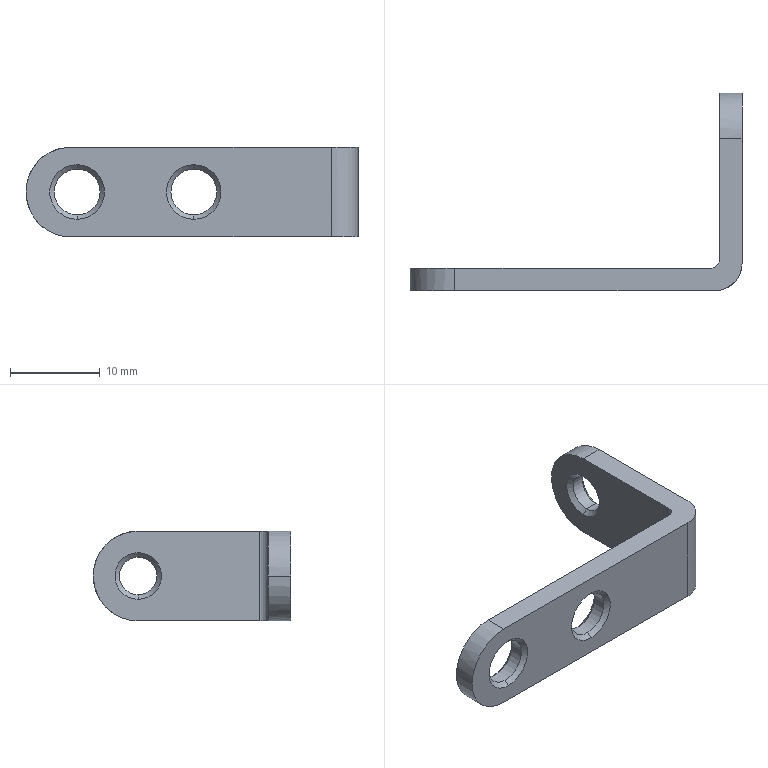Part | STEP file | 101000007811 | 1 solid | 30 faces | box 37 x 22 x 10 mm | volume 1193 mm3 | cone 12 | cylinder 12 | plane 6 | commonest cylinder face diameters 5.1 x4 10 x4 4.2 x2 2 x1 6 x1
STEP:
#1=CARTESIAN_POINT('',(-18.3,0.5,7.55));
#2=VERTEX_POINT('',#1);
#3=CARTESIAN_POINT('',(-20.85,0.5,5.));
#4=VERTEX_POINT('',#3);
#5=CARTESIAN_POINT('',(-18.3,0.5,5.));
#6=DIRECTION('',(0.,-1.,0.));
#7=AXIS2_PLACEMENT_3D('',#5,#6,$);
#8=CIRCLE('',#7,2.55);
#9=EDGE_CURVE('',#2,#4,#8,.T.);
#10=ORIENTED_EDGE('',*,*,#9,.F.);
#11=CARTESIAN_POINT('',(-18.3,0.,8.05));
#12=VERTEX_POINT('',#11);
#13=CARTESIAN_POINT('',(-18.3,-353551.866,353559.916));
#14=DIRECTION('',(0.,-0.7071,0.7071));
#15=VECTOR('',#14,1.);
#16=LINE('',#13,#15);
#17=EDGE_CURVE('',#2,#12,#16,.T.);
#18=ORIENTED_EDGE('',*,*,#17,.T.);
#19=CARTESIAN_POINT('',(-18.3,0.,1.95));
#20=VERTEX_POINT('',#19);
#21=CARTESIAN_POINT('',(-18.3,0.,5.));
#22=DIRECTION('',(0.,-1.,0.));
#23=AXIS2_PLACEMENT_3D('',#21,#22,$);
#24=CIRCLE('',#23,3.05);
#25=EDGE_CURVE('',#20,#12,#24,.F.);
#26=ORIENTED_EDGE('',*,*,#25,.F.);
#27=CARTESIAN_POINT('',(-18.3,0.5,2.45));
#28=VERTEX_POINT('',#27);
#29=CARTESIAN_POINT('',(-18.3,-353551.866,-353549.916));
#30=DIRECTION('',(0.,-0.7071,-0.7071));
#31=VECTOR('',#30,1.);
#32=LINE('',#29,#31);
#33=EDGE_CURVE('',#28,#20,#32,.T.);
#34=ORIENTED_EDGE('',*,*,#33,.F.);
#35=CARTESIAN_POINT('',(-18.3,0.5,5.));
#36=DIRECTION('',(0.,-1.,0.));
#37=AXIS2_PLACEMENT_3D('',#35,#36,$);
#38=CIRCLE('',#37,2.55);
#39=EDGE_CURVE('',#4,#28,#38,.T.);
#40=ORIENTED_EDGE('',*,*,#39,.F.);
#41=EDGE_LOOP('',(#10,#18,#26,#34,#40));
#42=FACE_OUTER_BOUND('',#41,.T.);
#43=CARTESIAN_POINT('',(-18.3,0.,5.));
#44=DIRECTION('',(0.,-1.,0.));
#45=DIRECTION('',(0.,0.,1.));
#46=AXIS2_PLACEMENT_3D('',#43,#44,#45);
#47=CONICAL_SURFACE('',#46,3.05,0.7854);
#48=ADVANCED_FACE('',(#42),#47,.F.);
#49=CARTESIAN_POINT('',(-15.75,0.5,5.));
#50=VERTEX_POINT('',#49);
#51=CARTESIAN_POINT('',(-15.75,2.,5.));
#52=VERTEX_POINT('',#51);
#53=CARTESIAN_POINT('',(-15.75,0.,5.));
#54=DIRECTION('',(0.,1.,0.));
#55=VECTOR('',#54,1.);
#56=LINE('',#53,#55);
#57=EDGE_CURVE('',#50,#52,#56,.T.);
#58=ORIENTED_EDGE('',*,*,#57,.F.);
#59=CARTESIAN_POINT('',(-18.3,0.5,5.));
#60=DIRECTION('',(0.,1.,0.));
#61=AXIS2_PLACEMENT_3D('',#59,#60,$);
#62=CIRCLE('',#61,2.55);
#63=EDGE_CURVE('',#50,#2,#62,.F.);
#64=ORIENTED_EDGE('',*,*,#63,.T.);
#65=ORIENTED_EDGE('',*,*,#9,.T.);
#66=CARTESIAN_POINT('',(-20.85,2.,5.));
#67=VERTEX_POINT('',#66);
#68=CARTESIAN_POINT('',(-20.85,0.,5.));
#69=DIRECTION('',(0.,1.,0.));
#70=VECTOR('',#69,1.);
#71=LINE('',#68,#70);
#72=EDGE_CURVE('',#4,#67,#71,.T.);
#73=ORIENTED_EDGE('',*,*,#72,.T.);
#74=CARTESIAN_POINT('',(-18.3,2.,7.55));
#75=VERTEX_POINT('',#74);
#76=CARTESIAN_POINT('',(-18.3,2.,5.));
#77=DIRECTION('',(0.,1.,0.));
#78=AXIS2_PLACEMENT_3D('',#76,#77,$);
#79=CIRCLE('',#78,2.55);
#80=EDGE_CURVE('',#67,#75,#79,.T.);
#81=ORIENTED_EDGE('',*,*,#80,.T.);
#82=CARTESIAN_POINT('',(-18.3,2.,5.));
#83=DIRECTION('',(0.,1.,0.));
#84=AXIS2_PLACEMENT_3D('',#82,#83,$);
#85=CIRCLE('',#84,2.55);
#86=EDGE_CURVE('',#75,#52,#85,.T.);
#87=ORIENTED_EDGE('',*,*,#86,.T.);
#88=EDGE_LOOP('',(#58,#64,#65,#73,#81,#87));
#89=FACE_OUTER_BOUND('',#88,.T.);
#90=CARTESIAN_POINT('',(-18.3,0.,5.));
#91=DIRECTION('',(0.,1.,0.));
#92=DIRECTION('',(-1.,0.,0.));
#93=AXIS2_PLACEMENT_3D('',#90,#91,#92);
#94=CYLINDRICAL_SURFACE('',#93,2.55);
#95=ADVANCED_FACE('',(#89),#94,.F.);
#96=ORIENTED_EDGE('',*,*,#17,.F.);
#97=ORIENTED_EDGE('',*,*,#63,.F.);
#98=CARTESIAN_POINT('',(-18.3,0.5,5.));
#99=DIRECTION('',(0.,-1.,0.));
#100=AXIS2_PLACEMENT_3D('',#98,#99,$);
#101=CIRCLE('',#100,2.55);
#102=EDGE_CURVE('',#28,#50,#101,.T.);
#103=ORIENTED_EDGE('',*,*,#102,.F.);
#104=ORIENTED_EDGE('',*,*,#33,.T.);
#105=CARTESIAN_POINT('',(-18.3,0.,5.));
#106=DIRECTION('',(0.,-1.,0.));
#107=AXIS2_PLACEMENT_3D('',#105,#106,$);
#108=CIRCLE('',#107,3.05);
#109=EDGE_CURVE('',#12,#20,#108,.F.);
#110=ORIENTED_EDGE('',*,*,#109,.F.);
#111=EDGE_LOOP('',(#96,#97,#103,#104,#110));
#112=FACE_OUTER_BOUND('',#111,.T.);
#113=CARTESIAN_POINT('',(-18.3,0.,5.));
#114=DIRECTION('',(0.,-1.,0.));
#115=DIRECTION('',(0.,0.,-1.));
#116=AXIS2_PLACEMENT_3D('',#113,#114,#115);
#117=CONICAL_SURFACE('',#116,3.05,0.7854);
#118=ADVANCED_FACE('',(#112),#117,.F.);
#119=CARTESIAN_POINT('',(-32.,0.,0.));
#120=VERTEX_POINT('',#119);
#121=CARTESIAN_POINT('',(-3.,0.,0.));
#122=VERTEX_POINT('',#121);
#123=CARTESIAN_POINT('',(-17.5,0.,0.));
#124=DIRECTION('',(1.,0.,0.));
#125=VECTOR('',#124,1.);
#126=LINE('',#123,#125);
#127=EDGE_CURVE('',#120,#122,#126,.T.);
#128=ORIENTED_EDGE('',*,*,#127,.T.);
#129=CARTESIAN_POINT('',(-3.,0.,10.));
#130=VERTEX_POINT('',#129);
#131=CARTESIAN_POINT('',(-3.,0.,5.));
#132=DIRECTION('',(0.,0.,1.));
#133=VECTOR('',#132,1.);
#134=LINE('',#131,#133);
#135=EDGE_CURVE('',#122,#130,#134,.T.);
#136=ORIENTED_EDGE('',*,*,#135,.T.);
#137=CARTESIAN_POINT('',(-32.,0.,10.));
#138=VERTEX_POINT('',#137);
#139=CARTESIAN_POINT('',(-17.5,0.,10.));
#140=DIRECTION('',(1.,0.,0.));
#141=VECTOR('',#140,1.);
#142=LINE('',#139,#141);
#143=EDGE_CURVE('',#138,#130,#142,.T.);
#144=ORIENTED_EDGE('',*,*,#143,.F.);
#145=CARTESIAN_POINT('',(-37.,0.,5.));
#146=VERTEX_POINT('',#145);
#147=CARTESIAN_POINT('',(-32.,0.,10.));
#148=CARTESIAN_POINT('',(-32.548,0.,10.));
#149=CARTESIAN_POINT('',(-33.095,0.,9.925));
#150=CARTESIAN_POINT('',(-33.629,0.,9.775));
#151=CARTESIAN_POINT('',(-34.643,0.,9.333));
#152=CARTESIAN_POINT('',(-35.5,0.,8.634));
#153=CARTESIAN_POINT('',(-35.878,0.,8.228));
#154=CARTESIAN_POINT('',(-36.47,0.,7.382));
#155=CARTESIAN_POINT('',(-36.831,0.,6.417));
#156=CARTESIAN_POINT('',(-36.944,0.,5.951));
#157=CARTESIAN_POINT('',(-37.,0.,5.475));
#158=CARTESIAN_POINT('',(-37.,0.,5.));
#159=B_SPLINE_CURVE_WITH_KNOTS('',5,(#147,#148,#149,#150,#151,#152,#153,#154,#155,#156,#157,#158),.UNSPECIFIED.,.F.,.U.,(6,3,3,6),(0.,3.873,7.746,11.107),.UNSPECIFIED.);
#160=EDGE_CURVE('',#138,#146,#159,.T.);
#161=ORIENTED_EDGE('',*,*,#160,.T.);
#162=CARTESIAN_POINT('',(-37.,0.,5.));
#163=CARTESIAN_POINT('',(-37.,0.,4.452));
#164=CARTESIAN_POINT('',(-36.925,0.,3.905));
#165=CARTESIAN_POINT('',(-36.775,0.,3.371));
#166=CARTESIAN_POINT('',(-36.333,0.,2.357));
#167=CARTESIAN_POINT('',(-35.634,0.,1.5));
#168=CARTESIAN_POINT('',(-35.228,0.,1.122));
#169=CARTESIAN_POINT('',(-34.382,0.,0.5296));
#170=CARTESIAN_POINT('',(-33.417,0.,0.1695));
#171=CARTESIAN_POINT('',(-32.951,0.,0.05649));
#172=CARTESIAN_POINT('',(-32.475,0.,0.));
#173=CARTESIAN_POINT('',(-32.,0.,0.));
#174=B_SPLINE_CURVE_WITH_KNOTS('',5,(#162,#163,#164,#165,#166,#167,#168,#169,#170,#171,#172,#173),.UNSPECIFIED.,.F.,.U.,(6,3,3,6),(0.,3.873,7.746,11.107),.UNSPECIFIED.);
#175=EDGE_CURVE('',#146,#120,#174,.T.);
#176=ORIENTED_EDGE('',*,*,#175,.T.);
#177=EDGE_LOOP('',(#128,#136,#144,#161,#176));
#178=FACE_OUTER_BOUND('',#177,.T.);
#179=CARTESIAN_POINT('',(-31.3,0.,1.95));
#180=VERTEX_POINT('',#179);
#181=CARTESIAN_POINT('',(-31.3,0.,8.05));
#182=VERTEX_POINT('',#181);
#183=CARTESIAN_POINT('',(-31.3,0.,5.));
#184=DIRECTION('',(0.,1.,0.));
#185=AXIS2_PLACEMENT_3D('',#183,#184,$);
#186=CIRCLE('',#185,3.05);
#187=EDGE_CURVE('',#180,#182,#186,.T.);
#188=ORIENTED_EDGE('',*,*,#187,.T.);
#189=CARTESIAN_POINT('',(-31.3,0.,5.));
#190=DIRECTION('',(0.,1.,0.));
#191=AXIS2_PLACEMENT_3D('',#189,#190,$);
#192=CIRCLE('',#191,3.05);
#193=EDGE_CURVE('',#182,#180,#192,.T.);
#194=ORIENTED_EDGE('',*,*,#193,.T.);
#195=EDGE_LOOP('',(#188,#194));
#196=FACE_BOUND('',#195,.T.);
#197=ORIENTED_EDGE('',*,*,#25,.T.);
#198=ORIENTED_EDGE('',*,*,#109,.T.);
#199=EDGE_LOOP('',(#197,#198));
#200=FACE_BOUND('',#199,.T.);
#201=CARTESIAN_POINT('',(0.,0.,10.));
#202=DIRECTION('',(0.,1.,0.));
#203=DIRECTION('',(-1.,0.,0.));
#204=AXIS2_PLACEMENT_3D('',#201,#202,#203);
#205=PLANE('',#204);
#206=ADVANCED_FACE('',(#178,#196,#200),#205,.F.);
#207=ORIENTED_EDGE('',*,*,#39,.T.);
#208=ORIENTED_EDGE('',*,*,#102,.T.);
#209=ORIENTED_EDGE('',*,*,#57,.T.);
#210=CARTESIAN_POINT('',(-18.3,2.,2.45));
#211=VERTEX_POINT('',#210);
#212=CARTESIAN_POINT('',(-18.3,2.,5.));
#213=DIRECTION('',(0.,1.,0.));
#214=AXIS2_PLACEMENT_3D('',#212,#213,$);
#215=CIRCLE('',#214,2.55);
#216=EDGE_CURVE('',#52,#211,#215,.T.);
#217=ORIENTED_EDGE('',*,*,#216,.T.);
#218=CARTESIAN_POINT('',(-18.3,2.,5.));
#219=DIRECTION('',(0.,1.,0.));
#220=AXIS2_PLACEMENT_3D('',#218,#219,$);
#221=CIRCLE('',#220,2.55);
#222=EDGE_CURVE('',#211,#67,#221,.T.);
#223=ORIENTED_EDGE('',*,*,#222,.T.);
#224=ORIENTED_EDGE('',*,*,#72,.F.);
#225=EDGE_LOOP('',(#207,#208,#209,#217,#223,#224));
#226=FACE_OUTER_BOUND('',#225,.T.);
#227=CARTESIAN_POINT('',(-18.3,0.,5.));
#228=DIRECTION('',(0.,1.,0.));
#229=DIRECTION('',(1.,0.,0.));
#230=AXIS2_PLACEMENT_3D('',#227,#228,#229);
#231=CYLINDRICAL_SURFACE('',#230,2.55);
#232=ADVANCED_FACE('',(#226),#231,.F.);
#233=ORIENTED_EDGE('',*,*,#222,.F.);
#234=CARTESIAN_POINT('',(-18.3,2.5,1.95));
#235=VERTEX_POINT('',#234);
#236=CARTESIAN_POINT('',(-18.3,353554.116,-353549.666));
#237=DIRECTION('',(0.,0.7071,-0.7071));
#238=VECTOR('',#237,1.);
#239=LINE('',#236,#238);
#240=EDGE_CURVE('',#211,#235,#239,.T.);
#241=ORIENTED_EDGE('',*,*,#240,.T.);
#242=CARTESIAN_POINT('',(-18.3,2.5,8.05));
#243=VERTEX_POINT('',#242);
#244=CARTESIAN_POINT('',(-18.3,2.5,5.));
#245=DIRECTION('',(0.,1.,0.));
#246=AXIS2_PLACEMENT_3D('',#244,#245,$);
#247=CIRCLE('',#246,3.05);
#248=EDGE_CURVE('',#243,#235,#247,.F.);
#249=ORIENTED_EDGE('',*,*,#248,.F.);
#250=CARTESIAN_POINT('',(-18.3,353554.116,353559.666));
#251=DIRECTION('',(0.,0.7071,0.7071));
#252=VECTOR('',#251,1.);
#253=LINE('',#250,#252);
#254=EDGE_CURVE('',#75,#243,#253,.T.);
#255=ORIENTED_EDGE('',*,*,#254,.F.);
#256=ORIENTED_EDGE('',*,*,#80,.F.);
#257=EDGE_LOOP('',(#233,#241,#249,#255,#256));
#258=FACE_OUTER_BOUND('',#257,.T.);
#259=CARTESIAN_POINT('',(-18.3,2.,5.));
#260=DIRECTION('',(0.,1.,0.));
#261=DIRECTION('',(0.,0.,-1.));
#262=AXIS2_PLACEMENT_3D('',#259,#260,#261);
#263=CONICAL_SURFACE('',#262,2.55,0.7854);
#264=ADVANCED_FACE('',(#258),#263,.F.);
#265=ORIENTED_EDGE('',*,*,#240,.F.);
#266=ORIENTED_EDGE('',*,*,#216,.F.);
#267=ORIENTED_EDGE('',*,*,#86,.F.);
#268=ORIENTED_EDGE('',*,*,#254,.T.);
#269=CARTESIAN_POINT('',(-18.3,2.5,5.));
#270=DIRECTION('',(0.,1.,0.));
#271=AXIS2_PLACEMENT_3D('',#269,#270,$);
#272=CIRCLE('',#271,3.05);
#273=EDGE_CURVE('',#235,#243,#272,.F.);
#274=ORIENTED_EDGE('',*,*,#273,.F.);
#275=EDGE_LOOP('',(#265,#266,#267,#268,#274));
#276=FACE_OUTER_BOUND('',#275,.T.);
#277=CARTESIAN_POINT('',(-18.3,2.,5.));
#278=DIRECTION('',(0.,1.,0.));
#279=DIRECTION('',(0.,0.,1.));
#280=AXIS2_PLACEMENT_3D('',#277,#278,#279);
#281=CONICAL_SURFACE('',#280,2.55,0.7854);
#282=ADVANCED_FACE('',(#276),#281,.F.);
#283=CARTESIAN_POINT('',(0.,3.,0.));
#284=VERTEX_POINT('',#283);
#285=CARTESIAN_POINT('',(0.,17.,0.));
#286=VERTEX_POINT('',#285);
#287=CARTESIAN_POINT('',(0.,10.,0.));
#288=DIRECTION('',(0.,1.,0.));
#289=VECTOR('',#288,1.);
#290=LINE('',#287,#289);
#291=EDGE_CURVE('',#284,#286,#290,.T.);
#292=ORIENTED_EDGE('',*,*,#291,.F.);
#293=CARTESIAN_POINT('',(0.,3.,0.));
#294=CARTESIAN_POINT('',(0.,2.661,0.));
#295=CARTESIAN_POINT('',(-0.048,2.321,0.));
#296=CARTESIAN_POINT('',(-0.144,1.991,0.));
#297=CARTESIAN_POINT('',(-0.4268,1.366,0.));
#298=CARTESIAN_POINT('',(-0.8717,0.8447,0.));
#299=CARTESIAN_POINT('',(-1.13,0.6172,0.));
#300=CARTESIAN_POINT('',(-1.639,0.2835,0.));
#301=CARTESIAN_POINT('',(-2.213,0.0869,0.));
#302=CARTESIAN_POINT('',(-2.473,0.02896,0.));
#303=CARTESIAN_POINT('',(-2.736,0.,0.));
#304=CARTESIAN_POINT('',(-3.,0.,0.));
#305=B_SPLINE_CURVE_WITH_KNOTS('',5,(#293,#294,#295,#296,#297,#298,#299,#300,#301,#302,#303,#304),.UNSPECIFIED.,.F.,.U.,(6,3,3,6),(0.,2.4,4.8,6.664),.UNSPECIFIED.);
#306=EDGE_CURVE('',#284,#122,#305,.T.);
#307=ORIENTED_EDGE('',*,*,#306,.T.);
#308=ORIENTED_EDGE('',*,*,#127,.F.);
#309=CARTESIAN_POINT('',(-32.,2.5,0.));
#310=VERTEX_POINT('',#309);
#311=CARTESIAN_POINT('',(-32.,1.25,0.));
#312=DIRECTION('',(0.,1.,0.));
#313=VECTOR('',#312,1.);
#314=LINE('',#311,#313);
#315=EDGE_CURVE('',#120,#310,#314,.T.);
#316=ORIENTED_EDGE('',*,*,#315,.T.);
#317=CARTESIAN_POINT('',(-3.5,2.5,0.));
#318=VERTEX_POINT('',#317);
#319=CARTESIAN_POINT('',(-17.75,2.5,0.));
#320=DIRECTION('',(-1.,0.,0.));
#321=VECTOR('',#320,1.);
#322=LINE('',#319,#321);
#323=EDGE_CURVE('',#318,#310,#322,.T.);
#324=ORIENTED_EDGE('',*,*,#323,.F.);
#325=CARTESIAN_POINT('',(-2.5,3.5,0.));
#326=VERTEX_POINT('',#325);
#327=CARTESIAN_POINT('',(-3.5,3.5,0.));
#328=DIRECTION('',(0.,0.,1.));
#329=AXIS2_PLACEMENT_3D('',#327,#328,$);
#330=CIRCLE('',#329,1.);
#331=EDGE_CURVE('',#318,#326,#330,.T.);
#332=ORIENTED_EDGE('',*,*,#331,.T.);
#333=CARTESIAN_POINT('',(-2.5,17.,0.));
#334=VERTEX_POINT('',#333);
#335=CARTESIAN_POINT('',(-2.5,10.25,0.));
#336=DIRECTION('',(0.,-1.,0.));
#337=VECTOR('',#336,1.);
#338=LINE('',#335,#337);
#339=EDGE_CURVE('',#334,#326,#338,.T.);
#340=ORIENTED_EDGE('',*,*,#339,.F.);
#341=CARTESIAN_POINT('',(-1.25,17.,0.));
#342=DIRECTION('',(1.,0.,0.));
#343=VECTOR('',#342,1.);
#344=LINE('',#341,#343);
#345=EDGE_CURVE('',#334,#286,#344,.T.);
#346=ORIENTED_EDGE('',*,*,#345,.T.);
#347=EDGE_LOOP('',(#292,#307,#308,#316,#324,#332,#340,#346));
#348=FACE_OUTER_BOUND('',#347,.T.);
#349=CARTESIAN_POINT('',(0.,0.,0.));
#350=DIRECTION('',(0.,0.,1.));
#351=DIRECTION('',(1.,0.,0.));
#352=AXIS2_PLACEMENT_3D('',#349,#350,#351);
#353=PLANE('',#352);
#354=ADVANCED_FACE('',(#348),#353,.F.);
#355=CARTESIAN_POINT('',(0.,3.,10.));
#356=VERTEX_POINT('',#355);
#357=CARTESIAN_POINT('',(-3.,3.,10.));
#358=DIRECTION('',(0.,0.,-1.));
#359=AXIS2_PLACEMENT_3D('',#357,#358,$);
#360=CIRCLE('',#359,3.);
#361=EDGE_CURVE('',#130,#356,#360,.F.);
#362=ORIENTED_EDGE('',*,*,#361,.F.);
#363=ORIENTED_EDGE('',*,*,#135,.F.);
#364=ORIENTED_EDGE('',*,*,#306,.F.);
#365=CARTESIAN_POINT('',(0.,3.,10.));
#366=DIRECTION('',(0.,0.,-1.));
#367=VECTOR('',#366,1.);
#368=LINE('',#365,#367);
#369=EDGE_CURVE('',#356,#284,#368,.T.);
#370=ORIENTED_EDGE('',*,*,#369,.F.);
#371=EDGE_LOOP('',(#362,#363,#364,#370));
#372=FACE_OUTER_BOUND('',#371,.T.);
#373=CARTESIAN_POINT('',(-3.,3.,10.));
#374=DIRECTION('',(0.,0.,-1.));
#375=DIRECTION('',(1.,0.,0.));
#376=AXIS2_PLACEMENT_3D('',#373,#374,#375);
#377=CYLINDRICAL_SURFACE('',#376,3.);
#378=ADVANCED_FACE('',(#372),#377,.T.);
#379=ORIENTED_EDGE('',*,*,#143,.T.);
#380=ORIENTED_EDGE('',*,*,#361,.T.);
#381=CARTESIAN_POINT('',(0.,17.,10.));
#382=VERTEX_POINT('',#381);
#383=CARTESIAN_POINT('',(0.,10.,10.));
#384=DIRECTION('',(0.,1.,0.));
#385=VECTOR('',#384,1.);
#386=LINE('',#383,#385);
#387=EDGE_CURVE('',#356,#382,#386,.T.);
#388=ORIENTED_EDGE('',*,*,#387,.T.);
#389=CARTESIAN_POINT('',(-2.5,17.,10.));
#390=VERTEX_POINT('',#389);
#391=CARTESIAN_POINT('',(-1.25,17.,10.));
#392=DIRECTION('',(-1.,0.,0.));
#393=VECTOR('',#392,1.);
#394=LINE('',#391,#393);
#395=EDGE_CURVE('',#382,#390,#394,.T.);
#396=ORIENTED_EDGE('',*,*,#395,.T.);
#397=CARTESIAN_POINT('',(-2.5,3.5,10.));
#398=VERTEX_POINT('',#397);
#399=CARTESIAN_POINT('',(-2.5,10.25,10.));
#400=DIRECTION('',(0.,-1.,0.));
#401=VECTOR('',#400,1.);
#402=LINE('',#399,#401);
#403=EDGE_CURVE('',#390,#398,#402,.T.);
#404=ORIENTED_EDGE('',*,*,#403,.T.);
#405=CARTESIAN_POINT('',(-3.5,2.5,10.));
#406=VERTEX_POINT('',#405);
#407=CARTESIAN_POINT('',(-2.5,3.5,10.));
#408=CARTESIAN_POINT('',(-2.5,3.402,10.));
#409=CARTESIAN_POINT('',(-2.512,3.304,10.));
#410=CARTESIAN_POINT('',(-2.536,3.208,10.));
#411=CARTESIAN_POINT('',(-2.607,3.024,10.));
#412=CARTESIAN_POINT('',(-2.72,2.862,10.));
#413=CARTESIAN_POINT('',(-2.787,2.789,10.));
#414=CARTESIAN_POINT('',(-2.936,2.66,10.));
#415=CARTESIAN_POINT('',(-3.112,2.57,10.));
#416=CARTESIAN_POINT('',(-3.205,2.537,10.));
#417=CARTESIAN_POINT('',(-3.321,2.51,10.));
#418=CARTESIAN_POINT('',(-3.439,2.502,10.));
#419=CARTESIAN_POINT('',(-3.46,2.501,10.));
#420=CARTESIAN_POINT('',(-3.48,2.5,10.));
#421=CARTESIAN_POINT('',(-3.5,2.5,10.));
#422=B_SPLINE_CURVE_WITH_KNOTS('',5,(#407,#408,#409,#410,#411,#412,#413,#414,#415,#416,#417,#418,#419,#420,#421),.UNSPECIFIED.,.F.,.U.,(6,3,3,3,6),(0.,0.6928,1.386,2.078,2.221),.UNSPECIFIED.);
#423=EDGE_CURVE('',#398,#406,#422,.T.);
#424=ORIENTED_EDGE('',*,*,#423,.T.);
#425=CARTESIAN_POINT('',(-32.,2.5,10.));
#426=VERTEX_POINT('',#425);
#427=CARTESIAN_POINT('',(-17.75,2.5,10.));
#428=DIRECTION('',(-1.,0.,0.));
#429=VECTOR('',#428,1.);
#430=LINE('',#427,#429);
#431=EDGE_CURVE('',#406,#426,#430,.T.);
#432=ORIENTED_EDGE('',*,*,#431,.T.);
#433=CARTESIAN_POINT('',(-32.,1.25,10.));
#434=DIRECTION('',(0.,-1.,0.));
#435=VECTOR('',#434,1.);
#436=LINE('',#433,#435);
#437=EDGE_CURVE('',#426,#138,#436,.T.);
#438=ORIENTED_EDGE('',*,*,#437,.T.);
#439=EDGE_LOOP('',(#379,#380,#388,#396,#404,#424,#432,#438));
#440=FACE_OUTER_BOUND('',#439,.T.);
#441=CARTESIAN_POINT('',(0.,0.,10.));
#442=DIRECTION('',(0.,0.,1.));
#443=DIRECTION('',(1.,0.,0.));
#444=AXIS2_PLACEMENT_3D('',#441,#442,#443);
#445=PLANE('',#444);
#446=ADVANCED_FACE('',(#440),#445,.T.);
#447=ORIENTED_EDGE('',*,*,#437,.F.);
#448=CARTESIAN_POINT('',(-37.,2.5,5.));
#449=VERTEX_POINT('',#448);
#450=CARTESIAN_POINT('',(-32.,2.5,5.));
#451=DIRECTION('',(0.,1.,0.));
#452=AXIS2_PLACEMENT_3D('',#450,#451,$);
#453=CIRCLE('',#452,5.);
#454=EDGE_CURVE('',#449,#426,#453,.T.);
#455=ORIENTED_EDGE('',*,*,#454,.F.);
#456=CARTESIAN_POINT('',(-37.,0.,5.));
#457=DIRECTION('',(0.,1.,0.));
#458=VECTOR('',#457,1.);
#459=LINE('',#456,#458);
#460=EDGE_CURVE('',#146,#449,#459,.T.);
#461=ORIENTED_EDGE('',*,*,#460,.F.);
#462=ORIENTED_EDGE('',*,*,#160,.F.);
#463=EDGE_LOOP('',(#447,#455,#461,#462));
#464=FACE_OUTER_BOUND('',#463,.T.);
#465=CARTESIAN_POINT('',(-32.,0.,5.));
#466=DIRECTION('',(0.,1.,0.));
#467=DIRECTION('',(0.,0.,-1.));
#468=AXIS2_PLACEMENT_3D('',#465,#466,#467);
#469=CYLINDRICAL_SURFACE('',#468,5.);
#470=ADVANCED_FACE('',(#464),#469,.T.);
#471=CARTESIAN_POINT('',(-32.,2.5,5.));
#472=DIRECTION('',(0.,-1.,0.));
#473=AXIS2_PLACEMENT_3D('',#471,#472,$);
#474=CIRCLE('',#473,5.);
#475=EDGE_CURVE('',#310,#449,#474,.F.);
#476=ORIENTED_EDGE('',*,*,#475,.F.);
#477=ORIENTED_EDGE('',*,*,#315,.F.);
#478=ORIENTED_EDGE('',*,*,#175,.F.);
#479=ORIENTED_EDGE('',*,*,#460,.T.);
#480=EDGE_LOOP('',(#476,#477,#478,#479));
#481=FACE_OUTER_BOUND('',#480,.T.);
#482=CARTESIAN_POINT('',(-32.,2.5,5.));
#483=DIRECTION('',(0.,-1.,0.));
#484=DIRECTION('',(0.,0.,1.));
#485=AXIS2_PLACEMENT_3D('',#482,#483,#484);
#486=CYLINDRICAL_SURFACE('',#485,5.);
#487=ADVANCED_FACE('',(#481),#486,.T.);
#488=CARTESIAN_POINT('',(-31.3,0.5,7.55));
#489=VERTEX_POINT('',#488);
#490=CARTESIAN_POINT('',(-33.85,0.5,5.));
#491=VERTEX_POINT('',#490);
#492=CARTESIAN_POINT('',(-31.3,0.5,5.));
#493=DIRECTION('',(0.,-1.,0.));
#494=AXIS2_PLACEMENT_3D('',#492,#493,$);
#495=CIRCLE('',#494,2.55);
#496=EDGE_CURVE('',#489,#491,#495,.T.);
#497=ORIENTED_EDGE('',*,*,#496,.F.);
#498=CARTESIAN_POINT('',(-31.3,-353551.866,353559.916));
#499=DIRECTION('',(0.,-0.7071,0.7071));
#500=VECTOR('',#499,1.);
#501=LINE('',#498,#500);
#502=EDGE_CURVE('',#489,#182,#501,.T.);
#503=ORIENTED_EDGE('',*,*,#502,.T.);
#504=ORIENTED_EDGE('',*,*,#187,.F.);
#505=CARTESIAN_POINT('',(-31.3,0.5,2.45));
#506=VERTEX_POINT('',#505);
#507=CARTESIAN_POINT('',(-31.3,-353551.866,-353549.916));
#508=DIRECTION('',(0.,-0.7071,-0.7071));
#509=VECTOR('',#508,1.);
#510=LINE('',#507,#509);
#511=EDGE_CURVE('',#506,#180,#510,.T.);
#512=ORIENTED_EDGE('',*,*,#511,.F.);
#513=CARTESIAN_POINT('',(-31.3,0.5,5.));
#514=DIRECTION('',(0.,-1.,0.));
#515=AXIS2_PLACEMENT_3D('',#513,#514,$);
#516=CIRCLE('',#515,2.55);
#517=EDGE_CURVE('',#491,#506,#516,.T.);
#518=ORIENTED_EDGE('',*,*,#517,.F.);
#519=EDGE_LOOP('',(#497,#503,#504,#512,#518));
#520=FACE_OUTER_BOUND('',#519,.T.);
#521=CARTESIAN_POINT('',(-31.3,0.,5.));
#522=DIRECTION('',(0.,-1.,0.));
#523=DIRECTION('',(0.,0.,1.));
#524=AXIS2_PLACEMENT_3D('',#521,#522,#523);
#525=CONICAL_SURFACE('',#524,3.05,0.7854);
#526=ADVANCED_FACE('',(#520),#525,.F.);
#527=ORIENTED_EDGE('',*,*,#502,.F.);
#528=CARTESIAN_POINT('',(-28.75,0.5,5.));
#529=VERTEX_POINT('',#528);
#530=CARTESIAN_POINT('',(-31.3,0.5,5.));
#531=DIRECTION('',(0.,-1.,0.));
#532=AXIS2_PLACEMENT_3D('',#530,#531,$);
#533=CIRCLE('',#532,2.55);
#534=EDGE_CURVE('',#529,#489,#533,.T.);
#535=ORIENTED_EDGE('',*,*,#534,.F.);
#536=CARTESIAN_POINT('',(-31.3,0.5,5.));
#537=DIRECTION('',(0.,-1.,0.));
#538=AXIS2_PLACEMENT_3D('',#536,#537,$);
#539=CIRCLE('',#538,2.55);
#540=EDGE_CURVE('',#506,#529,#539,.T.);
#541=ORIENTED_EDGE('',*,*,#540,.F.);
#542=ORIENTED_EDGE('',*,*,#511,.T.);
#543=ORIENTED_EDGE('',*,*,#193,.F.);
#544=EDGE_LOOP('',(#527,#535,#541,#542,#543));
#545=FACE_OUTER_BOUND('',#544,.T.);
#546=CARTESIAN_POINT('',(-31.3,0.,5.));
#547=DIRECTION('',(0.,-1.,0.));
#548=DIRECTION('',(0.,0.,-1.));
#549=AXIS2_PLACEMENT_3D('',#546,#547,#548);
#550=CONICAL_SURFACE('',#549,3.05,0.7854);
#551=ADVANCED_FACE('',(#545),#550,.F.);
#552=ORIENTED_EDGE('',*,*,#431,.F.);
#553=CARTESIAN_POINT('',(-3.5,2.5,5.));
#554=DIRECTION('',(0.,0.,-1.));
#555=VECTOR('',#554,1.);
#556=LINE('',#553,#555);
#557=EDGE_CURVE('',#406,#318,#556,.T.);
#558=ORIENTED_EDGE('',*,*,#557,.T.);
#559=ORIENTED_EDGE('',*,*,#323,.T.);
#560=ORIENTED_EDGE('',*,*,#475,.T.);
#561=ORIENTED_EDGE('',*,*,#454,.T.);
#562=EDGE_LOOP('',(#552,#558,#559,#560,#561));
#563=FACE_OUTER_BOUND('',#562,.T.);
#564=CARTESIAN_POINT('',(-31.3,2.5,8.05));
#565=VERTEX_POINT('',#564);
#566=CARTESIAN_POINT('',(-31.3,2.5,1.95));
#567=VERTEX_POINT('',#566);
#568=CARTESIAN_POINT('',(-31.3,2.5,5.));
#569=DIRECTION('',(0.,-1.,0.));
#570=AXIS2_PLACEMENT_3D('',#568,#569,$);
#571=CIRCLE('',#570,3.05);
#572=EDGE_CURVE('',#565,#567,#571,.T.);
#573=ORIENTED_EDGE('',*,*,#572,.T.);
#574=CARTESIAN_POINT('',(-31.3,2.5,5.));
#575=DIRECTION('',(0.,-1.,0.));
#576=AXIS2_PLACEMENT_3D('',#574,#575,$);
#577=CIRCLE('',#576,3.05);
#578=EDGE_CURVE('',#567,#565,#577,.T.);
#579=ORIENTED_EDGE('',*,*,#578,.T.);
#580=EDGE_LOOP('',(#573,#579));
#581=FACE_BOUND('',#580,.T.);
#582=ORIENTED_EDGE('',*,*,#248,.T.);
#583=ORIENTED_EDGE('',*,*,#273,.T.);
#584=EDGE_LOOP('',(#582,#583));
#585=FACE_BOUND('',#584,.T.);
#586=CARTESIAN_POINT('',(-2.5,2.5,10.));
#587=DIRECTION('',(0.,-1.,0.));
#588=DIRECTION('',(1.,0.,0.));
#589=AXIS2_PLACEMENT_3D('',#586,#587,#588);
#590=PLANE('',#589);
#591=ADVANCED_FACE('',(#563,#581,#585),#590,.F.);
#592=ORIENTED_EDGE('',*,*,#387,.F.);
#593=ORIENTED_EDGE('',*,*,#369,.T.);
#594=ORIENTED_EDGE('',*,*,#291,.T.);
#595=CARTESIAN_POINT('',(0.,22.,5.));
#596=VERTEX_POINT('',#595);
#597=CARTESIAN_POINT('',(0.,17.,0.));
#598=CARTESIAN_POINT('',(0.,17.548,0.));
#599=CARTESIAN_POINT('',(0.,18.095,0.075));
#600=CARTESIAN_POINT('',(0.,18.629,0.225));
#601=CARTESIAN_POINT('',(0.,19.643,0.6674));
#602=CARTESIAN_POINT('',(0.,20.5,1.366));
#603=CARTESIAN_POINT('',(0.,20.878,1.772));
#604=CARTESIAN_POINT('',(0.,21.47,2.618));
#605=CARTESIAN_POINT('',(0.,21.831,3.583));
#606=CARTESIAN_POINT('',(0.,21.944,4.049));
#607=CARTESIAN_POINT('',(0.,22.,4.525));
#608=CARTESIAN_POINT('',(0.,22.,5.));
#609=B_SPLINE_CURVE_WITH_KNOTS('',5,(#597,#598,#599,#600,#601,#602,#603,#604,#605,#606,#607,#608),.UNSPECIFIED.,.F.,.U.,(6,3,3,6),(0.,3.873,7.746,11.107),.UNSPECIFIED.);
#610=EDGE_CURVE('',#286,#596,#609,.T.);
#611=ORIENTED_EDGE('',*,*,#610,.T.);
#612=CARTESIAN_POINT('',(0.,22.,5.));
#613=CARTESIAN_POINT('',(0.,22.,5.548));
#614=CARTESIAN_POINT('',(0.,21.925,6.095));
#615=CARTESIAN_POINT('',(0.,21.775,6.629));
#616=CARTESIAN_POINT('',(0.,21.333,7.643));
#617=CARTESIAN_POINT('',(0.,20.634,8.5));
#618=CARTESIAN_POINT('',(0.,20.228,8.878));
#619=CARTESIAN_POINT('',(0.,19.382,9.47));
#620=CARTESIAN_POINT('',(0.,18.417,9.831));
#621=CARTESIAN_POINT('',(0.,17.951,9.944));
#622=CARTESIAN_POINT('',(0.,17.475,10.));
#623=CARTESIAN_POINT('',(0.,17.,10.));
#624=B_SPLINE_CURVE_WITH_KNOTS('',5,(#612,#613,#614,#615,#616,#617,#618,#619,#620,#621,#622,#623),.UNSPECIFIED.,.F.,.U.,(6,3,3,6),(0.,3.873,7.746,11.107),.UNSPECIFIED.);
#625=EDGE_CURVE('',#596,#382,#624,.T.);
#626=ORIENTED_EDGE('',*,*,#625,.T.);
#627=EDGE_LOOP('',(#592,#593,#594,#611,#626));
#628=FACE_OUTER_BOUND('',#627,.T.);
#629=CARTESIAN_POINT('',(0.,17.,2.4));
#630=VERTEX_POINT('',#629);
#631=CARTESIAN_POINT('',(0.,17.,7.6));
#632=VERTEX_POINT('',#631);
#633=CARTESIAN_POINT('',(0.,17.,5.));
#634=DIRECTION('',(-1.,0.,0.));
#635=AXIS2_PLACEMENT_3D('',#633,#634,$);
#636=CIRCLE('',#635,2.6);
#637=EDGE_CURVE('',#630,#632,#636,.T.);
#638=ORIENTED_EDGE('',*,*,#637,.T.);
#639=CARTESIAN_POINT('',(0.,17.,5.));
#640=DIRECTION('',(-1.,0.,0.));
#641=AXIS2_PLACEMENT_3D('',#639,#640,$);
#642=CIRCLE('',#641,2.6);
#643=EDGE_CURVE('',#632,#630,#642,.T.);
#644=ORIENTED_EDGE('',*,*,#643,.T.);
#645=EDGE_LOOP('',(#638,#644));
#646=FACE_BOUND('',#645,.T.);
#647=CARTESIAN_POINT('',(0.,0.,10.));
#648=DIRECTION('',(-1.,0.,0.));
#649=DIRECTION('',(0.,0.,1.));
#650=AXIS2_PLACEMENT_3D('',#647,#648,#649);
#651=PLANE('',#650);
#652=ADVANCED_FACE('',(#628,#646),#651,.F.);
#653=ORIENTED_EDGE('',*,*,#423,.F.);
#654=CARTESIAN_POINT('',(-2.5,3.5,10.));
#655=DIRECTION('',(0.,0.,1.));
#656=VECTOR('',#655,1.);
#657=LINE('',#654,#656);
#658=EDGE_CURVE('',#326,#398,#657,.T.);
#659=ORIENTED_EDGE('',*,*,#658,.F.);
#660=ORIENTED_EDGE('',*,*,#331,.F.);
#661=ORIENTED_EDGE('',*,*,#557,.F.);
#662=EDGE_LOOP('',(#653,#659,#660,#661));
#663=FACE_OUTER_BOUND('',#662,.T.);
#664=CARTESIAN_POINT('',(-3.5,3.5,10.));
#665=DIRECTION('',(0.,0.,1.));
#666=DIRECTION('',(-1.,0.,0.));
#667=AXIS2_PLACEMENT_3D('',#664,#665,#666);
#668=CYLINDRICAL_SURFACE('',#667,1.);
#669=ADVANCED_FACE('',(#663),#668,.F.);
#670=ORIENTED_EDGE('',*,*,#339,.T.);
#671=ORIENTED_EDGE('',*,*,#658,.T.);
#672=ORIENTED_EDGE('',*,*,#403,.F.);
#673=CARTESIAN_POINT('',(-2.5,22.,5.));
#674=VERTEX_POINT('',#673);
#675=CARTESIAN_POINT('',(-2.5,17.,10.));
#676=CARTESIAN_POINT('',(-2.5,17.548,10.));
#677=CARTESIAN_POINT('',(-2.5,18.095,9.925));
#678=CARTESIAN_POINT('',(-2.5,18.629,9.775));
#679=CARTESIAN_POINT('',(-2.5,19.643,9.333));
#680=CARTESIAN_POINT('',(-2.5,20.5,8.634));
#681=CARTESIAN_POINT('',(-2.5,20.878,8.228));
#682=CARTESIAN_POINT('',(-2.5,21.47,7.382));
#683=CARTESIAN_POINT('',(-2.5,21.831,6.417));
#684=CARTESIAN_POINT('',(-2.5,21.944,5.951));
#685=CARTESIAN_POINT('',(-2.5,22.,5.475));
#686=CARTESIAN_POINT('',(-2.5,22.,5.));
#687=B_SPLINE_CURVE_WITH_KNOTS('',5,(#675,#676,#677,#678,#679,#680,#681,#682,#683,#684,#685,#686),.UNSPECIFIED.,.F.,.U.,(6,3,3,6),(0.,3.873,7.746,11.107),.UNSPECIFIED.);
#688=EDGE_CURVE('',#390,#674,#687,.T.);
#689=ORIENTED_EDGE('',*,*,#688,.T.);
#690=CARTESIAN_POINT('',(-2.5,22.,5.));
#691=CARTESIAN_POINT('',(-2.5,22.,4.452));
#692=CARTESIAN_POINT('',(-2.5,21.925,3.905));
#693=CARTESIAN_POINT('',(-2.5,21.775,3.371));
#694=CARTESIAN_POINT('',(-2.5,21.333,2.357));
#695=CARTESIAN_POINT('',(-2.5,20.634,1.5));
#696=CARTESIAN_POINT('',(-2.5,20.228,1.122));
#697=CARTESIAN_POINT('',(-2.5,19.382,0.5296));
#698=CARTESIAN_POINT('',(-2.5,18.417,0.1695));
#699=CARTESIAN_POINT('',(-2.5,17.951,0.05649));
#700=CARTESIAN_POINT('',(-2.5,17.475,0.));
#701=CARTESIAN_POINT('',(-2.5,17.,0.));
#702=B_SPLINE_CURVE_WITH_KNOTS('',5,(#690,#691,#692,#693,#694,#695,#696,#697,#698,#699,#700,#701),.UNSPECIFIED.,.F.,.U.,(6,3,3,6),(0.,3.873,7.746,11.107),.UNSPECIFIED.);
#703=EDGE_CURVE('',#674,#334,#702,.T.);
#704=ORIENTED_EDGE('',*,*,#703,.T.);
#705=EDGE_LOOP('',(#670,#671,#672,#689,#704));
#706=FACE_OUTER_BOUND('',#705,.T.);
#707=CARTESIAN_POINT('',(-2.5,17.,7.6));
#708=VERTEX_POINT('',#707);
#709=CARTESIAN_POINT('',(-2.5,17.,2.4));
#710=VERTEX_POINT('',#709);
#711=CARTESIAN_POINT('',(-2.5,17.,5.));
#712=DIRECTION('',(1.,0.,0.));
#713=AXIS2_PLACEMENT_3D('',#711,#712,$);
#714=CIRCLE('',#713,2.6);
#715=EDGE_CURVE('',#708,#710,#714,.T.);
#716=ORIENTED_EDGE('',*,*,#715,.T.);
#717=CARTESIAN_POINT('',(-2.5,17.,5.));
#718=DIRECTION('',(1.,0.,0.));
#719=AXIS2_PLACEMENT_3D('',#717,#718,$);
#720=CIRCLE('',#719,2.6);
#721=EDGE_CURVE('',#710,#708,#720,.T.);
#722=ORIENTED_EDGE('',*,*,#721,.T.);
#723=EDGE_LOOP('',(#716,#722));
#724=FACE_BOUND('',#723,.T.);
#725=CARTESIAN_POINT('',(-2.5,2.5,10.));
#726=DIRECTION('',(1.,0.,0.));
#727=DIRECTION('',(0.,0.,-1.));
#728=AXIS2_PLACEMENT_3D('',#725,#726,#727);
#729=PLANE('',#728);
#730=ADVANCED_FACE('',(#706,#724),#729,.F.);
#731=ORIENTED_EDGE('',*,*,#610,.F.);
#732=ORIENTED_EDGE('',*,*,#345,.F.);
#733=ORIENTED_EDGE('',*,*,#703,.F.);
#734=CARTESIAN_POINT('',(-2.5,22.,5.));
#735=DIRECTION('',(-1.,0.,0.));
#736=VECTOR('',#735,1.);
#737=LINE('',#734,#736);
#738=EDGE_CURVE('',#674,#596,#737,.F.);
#739=ORIENTED_EDGE('',*,*,#738,.T.);
#740=EDGE_LOOP('',(#731,#732,#733,#739));
#741=FACE_OUTER_BOUND('',#740,.T.);
#742=CARTESIAN_POINT('',(-2.5,17.,5.));
#743=DIRECTION('',(-1.,0.,0.));
#744=DIRECTION('',(0.,0.,1.));
#745=AXIS2_PLACEMENT_3D('',#742,#743,#744);
#746=CYLINDRICAL_SURFACE('',#745,5.);
#747=ADVANCED_FACE('',(#741),#746,.T.);
#748=ORIENTED_EDGE('',*,*,#395,.F.);
#749=ORIENTED_EDGE('',*,*,#625,.F.);
#750=ORIENTED_EDGE('',*,*,#738,.F.);
#751=ORIENTED_EDGE('',*,*,#688,.F.);
#752=EDGE_LOOP('',(#748,#749,#750,#751));
#753=FACE_OUTER_BOUND('',#752,.T.);
#754=CARTESIAN_POINT('',(0.,17.,5.));
#755=DIRECTION('',(1.,0.,0.));
#756=DIRECTION('',(0.,0.,-1.));
#757=AXIS2_PLACEMENT_3D('',#754,#755,#756);
#758=CYLINDRICAL_SURFACE('',#757,5.);
#759=ADVANCED_FACE('',(#753),#758,.T.);
#760=CARTESIAN_POINT('',(-28.75,2.,5.));
#761=VERTEX_POINT('',#760);
#762=CARTESIAN_POINT('',(-28.75,0.,5.));
#763=DIRECTION('',(0.,1.,0.));
#764=VECTOR('',#763,1.);
#765=LINE('',#762,#764);
#766=EDGE_CURVE('',#529,#761,#765,.T.);
#767=ORIENTED_EDGE('',*,*,#766,.F.);
#768=ORIENTED_EDGE('',*,*,#534,.T.);
#769=ORIENTED_EDGE('',*,*,#496,.T.);
#770=CARTESIAN_POINT('',(-33.85,2.,5.));
#771=VERTEX_POINT('',#770);
#772=CARTESIAN_POINT('',(-33.85,0.,5.));
#773=DIRECTION('',(0.,1.,0.));
#774=VECTOR('',#773,1.);
#775=LINE('',#772,#774);
#776=EDGE_CURVE('',#491,#771,#775,.T.);
#777=ORIENTED_EDGE('',*,*,#776,.T.);
#778=CARTESIAN_POINT('',(-31.3,2.,7.55));
#779=VERTEX_POINT('',#778);
#780=CARTESIAN_POINT('',(-31.3,2.,5.));
#781=DIRECTION('',(0.,1.,0.));
#782=AXIS2_PLACEMENT_3D('',#780,#781,$);
#783=CIRCLE('',#782,2.55);
#784=EDGE_CURVE('',#771,#779,#783,.T.);
#785=ORIENTED_EDGE('',*,*,#784,.T.);
#786=CARTESIAN_POINT('',(-31.3,2.,5.));
#787=DIRECTION('',(0.,1.,0.));
#788=AXIS2_PLACEMENT_3D('',#786,#787,$);
#789=CIRCLE('',#788,2.55);
#790=EDGE_CURVE('',#779,#761,#789,.T.);
#791=ORIENTED_EDGE('',*,*,#790,.T.);
#792=EDGE_LOOP('',(#767,#768,#769,#777,#785,#791));
#793=FACE_OUTER_BOUND('',#792,.T.);
#794=CARTESIAN_POINT('',(-31.3,0.,5.));
#795=DIRECTION('',(0.,1.,0.));
#796=DIRECTION('',(-1.,0.,0.));
#797=AXIS2_PLACEMENT_3D('',#794,#795,#796);
#798=CYLINDRICAL_SURFACE('',#797,2.55);
#799=ADVANCED_FACE('',(#793),#798,.F.);
#800=ORIENTED_EDGE('',*,*,#517,.T.);
#801=ORIENTED_EDGE('',*,*,#540,.T.);
#802=ORIENTED_EDGE('',*,*,#766,.T.);
#803=CARTESIAN_POINT('',(-31.3,2.,2.45));
#804=VERTEX_POINT('',#803);
#805=CARTESIAN_POINT('',(-31.3,2.,5.));
#806=DIRECTION('',(0.,1.,0.));
#807=AXIS2_PLACEMENT_3D('',#805,#806,$);
#808=CIRCLE('',#807,2.55);
#809=EDGE_CURVE('',#761,#804,#808,.T.);
#810=ORIENTED_EDGE('',*,*,#809,.T.);
#811=CARTESIAN_POINT('',(-31.3,2.,5.));
#812=DIRECTION('',(0.,1.,0.));
#813=AXIS2_PLACEMENT_3D('',#811,#812,$);
#814=CIRCLE('',#813,2.55);
#815=EDGE_CURVE('',#804,#771,#814,.T.);
#816=ORIENTED_EDGE('',*,*,#815,.T.);
#817=ORIENTED_EDGE('',*,*,#776,.F.);
#818=EDGE_LOOP('',(#800,#801,#802,#810,#816,#817));
#819=FACE_OUTER_BOUND('',#818,.T.);
#820=CARTESIAN_POINT('',(-31.3,0.,5.));
#821=DIRECTION('',(0.,1.,0.));
#822=DIRECTION('',(1.,0.,0.));
#823=AXIS2_PLACEMENT_3D('',#820,#821,#822);
#824=CYLINDRICAL_SURFACE('',#823,2.55);
#825=ADVANCED_FACE('',(#819),#824,.F.);
#826=ORIENTED_EDGE('',*,*,#815,.F.);
#827=CARTESIAN_POINT('',(-31.3,353554.116,-353549.666));
#828=DIRECTION('',(0.,0.7071,-0.7071));
#829=VECTOR('',#828,1.);
#830=LINE('',#827,#829);
#831=EDGE_CURVE('',#804,#567,#830,.T.);
#832=ORIENTED_EDGE('',*,*,#831,.T.);
#833=ORIENTED_EDGE('',*,*,#572,.F.);
#834=CARTESIAN_POINT('',(-31.3,353554.116,353559.666));
#835=DIRECTION('',(0.,0.7071,0.7071));
#836=VECTOR('',#835,1.);
#837=LINE('',#834,#836);
#838=EDGE_CURVE('',#779,#565,#837,.T.);
#839=ORIENTED_EDGE('',*,*,#838,.F.);
#840=ORIENTED_EDGE('',*,*,#784,.F.);
#841=EDGE_LOOP('',(#826,#832,#833,#839,#840));
#842=FACE_OUTER_BOUND('',#841,.T.);
#843=CARTESIAN_POINT('',(-31.3,2.,5.));
#844=DIRECTION('',(0.,1.,0.));
#845=DIRECTION('',(0.,0.,-1.));
#846=AXIS2_PLACEMENT_3D('',#843,#844,#845);
#847=CONICAL_SURFACE('',#846,2.55,0.7854);
#848=ADVANCED_FACE('',(#842),#847,.F.);
#849=ORIENTED_EDGE('',*,*,#831,.F.);
#850=ORIENTED_EDGE('',*,*,#809,.F.);
#851=ORIENTED_EDGE('',*,*,#790,.F.);
#852=ORIENTED_EDGE('',*,*,#838,.T.);
#853=ORIENTED_EDGE('',*,*,#578,.F.);
#854=EDGE_LOOP('',(#849,#850,#851,#852,#853));
#855=FACE_OUTER_BOUND('',#854,.T.);
#856=CARTESIAN_POINT('',(-31.3,2.,5.));
#857=DIRECTION('',(0.,1.,0.));
#858=DIRECTION('',(0.,0.,1.));
#859=AXIS2_PLACEMENT_3D('',#856,#857,#858);
#860=CONICAL_SURFACE('',#859,2.55,0.7854);
#861=ADVANCED_FACE('',(#855),#860,.F.);
#862=CARTESIAN_POINT('',(-0.5,17.,7.1));
#863=VERTEX_POINT('',#862);
#864=CARTESIAN_POINT('',(-0.5,17.,2.9));
#865=VERTEX_POINT('',#864);
#866=CARTESIAN_POINT('',(-0.5,17.,5.));
#867=DIRECTION('',(1.,0.,0.));
#868=AXIS2_PLACEMENT_3D('',#866,#867,$);
#869=CIRCLE('',#868,2.1);
#870=EDGE_CURVE('',#863,#865,#869,.T.);
#871=ORIENTED_EDGE('',*,*,#870,.F.);
#872=CARTESIAN_POINT('',(353552.091,17.,353559.691));
#873=DIRECTION('',(0.7071,0.,0.7071));
#874=VECTOR('',#873,1.);
#875=LINE('',#872,#874);
#876=EDGE_CURVE('',#863,#632,#875,.T.);
#877=ORIENTED_EDGE('',*,*,#876,.T.);
#878=ORIENTED_EDGE('',*,*,#637,.F.);
#879=CARTESIAN_POINT('',(353552.091,17.,-353549.691));
#880=DIRECTION('',(0.7071,0.,-0.7071));
#881=VECTOR('',#880,1.);
#882=LINE('',#879,#881);
#883=EDGE_CURVE('',#865,#630,#882,.T.);
#884=ORIENTED_EDGE('',*,*,#883,.F.);
#885=EDGE_LOOP('',(#871,#877,#878,#884));
#886=FACE_OUTER_BOUND('',#885,.T.);
#887=CARTESIAN_POINT('',(0.,17.,5.));
#888=DIRECTION('',(1.,0.,0.));
#889=DIRECTION('',(0.,0.,1.));
#890=AXIS2_PLACEMENT_3D('',#887,#888,#889);
#891=CONICAL_SURFACE('',#890,2.6,0.7854);
#892=ADVANCED_FACE('',(#886),#891,.F.);
#893=ORIENTED_EDGE('',*,*,#876,.F.);
#894=CARTESIAN_POINT('',(-0.5,17.,5.));
#895=DIRECTION('',(1.,0.,0.));
#896=AXIS2_PLACEMENT_3D('',#894,#895,$);
#897=CIRCLE('',#896,2.1);
#898=EDGE_CURVE('',#865,#863,#897,.T.);
#899=ORIENTED_EDGE('',*,*,#898,.F.);
#900=ORIENTED_EDGE('',*,*,#883,.T.);
#901=ORIENTED_EDGE('',*,*,#643,.F.);
#902=EDGE_LOOP('',(#893,#899,#900,#901));
#903=FACE_OUTER_BOUND('',#902,.T.);
#904=CARTESIAN_POINT('',(0.,17.,5.));
#905=DIRECTION('',(1.,0.,0.));
#906=DIRECTION('',(0.,0.,-1.));
#907=AXIS2_PLACEMENT_3D('',#904,#905,#906);
#908=CONICAL_SURFACE('',#907,2.6,0.7854);
#909=ADVANCED_FACE('',(#903),#908,.F.);
#910=CARTESIAN_POINT('',(-2.,17.,2.9));
#911=VERTEX_POINT('',#910);
#912=CARTESIAN_POINT('',(-2.,17.,7.1));
#913=VERTEX_POINT('',#912);
#914=CARTESIAN_POINT('',(-2.,17.,5.));
#915=DIRECTION('',(-1.,0.,0.));
#916=AXIS2_PLACEMENT_3D('',#914,#915,$);
#917=CIRCLE('',#916,2.1);
#918=EDGE_CURVE('',#911,#913,#917,.T.);
#919=ORIENTED_EDGE('',*,*,#918,.F.);
#920=CARTESIAN_POINT('',(-353554.341,17.,-353549.441));
#921=DIRECTION('',(-0.7071,0.,-0.7071));
#922=VECTOR('',#921,1.);
#923=LINE('',#920,#922);
#924=EDGE_CURVE('',#911,#710,#923,.T.);
#925=ORIENTED_EDGE('',*,*,#924,.T.);
#926=ORIENTED_EDGE('',*,*,#715,.F.);
#927=CARTESIAN_POINT('',(-353554.341,17.,353559.441));
#928=DIRECTION('',(-0.7071,0.,0.7071));
#929=VECTOR('',#928,1.);
#930=LINE('',#927,#929);
#931=EDGE_CURVE('',#913,#708,#930,.T.);
#932=ORIENTED_EDGE('',*,*,#931,.F.);
#933=EDGE_LOOP('',(#919,#925,#926,#932));
#934=FACE_OUTER_BOUND('',#933,.T.);
#935=CARTESIAN_POINT('',(-2.,17.,5.));
#936=DIRECTION('',(-1.,0.,0.));
#937=DIRECTION('',(0.,0.,-1.));
#938=AXIS2_PLACEMENT_3D('',#935,#936,#937);
#939=CONICAL_SURFACE('',#938,2.1,0.7854);
#940=ADVANCED_FACE('',(#934),#939,.F.);
#941=ORIENTED_EDGE('',*,*,#924,.F.);
#942=CARTESIAN_POINT('',(-2.,17.,5.));
#943=DIRECTION('',(-1.,0.,0.));
#944=AXIS2_PLACEMENT_3D('',#942,#943,$);
#945=CIRCLE('',#944,2.1);
#946=EDGE_CURVE('',#913,#911,#945,.T.);
#947=ORIENTED_EDGE('',*,*,#946,.F.);
#948=ORIENTED_EDGE('',*,*,#931,.T.);
#949=ORIENTED_EDGE('',*,*,#721,.F.);
#950=EDGE_LOOP('',(#941,#947,#948,#949));
#951=FACE_OUTER_BOUND('',#950,.T.);
#952=CARTESIAN_POINT('',(-2.,17.,5.));
#953=DIRECTION('',(-1.,0.,0.));
#954=DIRECTION('',(0.,0.,1.));
#955=AXIS2_PLACEMENT_3D('',#952,#953,#954);
#956=CONICAL_SURFACE('',#955,2.1,0.7854);
#957=ADVANCED_FACE('',(#951),#956,.F.);
#958=ORIENTED_EDGE('',*,*,#870,.T.);
#959=CARTESIAN_POINT('',(0.,17.,2.9));
#960=DIRECTION('',(-1.,0.,0.));
#961=VECTOR('',#960,1.);
#962=LINE('',#959,#961);
#963=EDGE_CURVE('',#865,#911,#962,.T.);
#964=ORIENTED_EDGE('',*,*,#963,.T.);
#965=ORIENTED_EDGE('',*,*,#918,.T.);
#966=CARTESIAN_POINT('',(0.,17.,7.1));
#967=DIRECTION('',(-1.,0.,0.));
#968=VECTOR('',#967,1.);
#969=LINE('',#966,#968);
#970=EDGE_CURVE('',#863,#913,#969,.T.);
#971=ORIENTED_EDGE('',*,*,#970,.F.);
#972=EDGE_LOOP('',(#958,#964,#965,#971));
#973=FACE_OUTER_BOUND('',#972,.T.);
#974=CARTESIAN_POINT('',(0.,17.,5.));
#975=DIRECTION('',(-1.,0.,0.));
#976=DIRECTION('',(0.,0.,-1.));
#977=AXIS2_PLACEMENT_3D('',#974,#975,#976);
#978=CYLINDRICAL_SURFACE('',#977,2.1);
#979=ADVANCED_FACE('',(#973),#978,.F.);
#980=ORIENTED_EDGE('',*,*,#963,.F.);
#981=ORIENTED_EDGE('',*,*,#898,.T.);
#982=ORIENTED_EDGE('',*,*,#970,.T.);
#983=ORIENTED_EDGE('',*,*,#946,.T.);
#984=EDGE_LOOP('',(#980,#981,#982,#983));
#985=FACE_OUTER_BOUND('',#984,.T.);
#986=CARTESIAN_POINT('',(0.,17.,5.));
#987=DIRECTION('',(-1.,0.,0.));
#988=DIRECTION('',(0.,0.,1.));
#989=AXIS2_PLACEMENT_3D('',#986,#987,#988);
#990=CYLINDRICAL_SURFACE('',#989,2.1);
#991=ADVANCED_FACE('',(#985),#990,.F.);
#992=CLOSED_SHELL('',(#48,#95,#118,#206,#232,#264,#282,#354,#378,#446,#470,#487,#526,#551,#591,#652,#669,#730,#747,#759,#799,#825,#848,#861,#892,#909,#940,#957,#979,#991));
#993=MANIFOLD_SOLID_BREP('',#992);
#994=(LENGTH_UNIT()NAMED_UNIT(*)SI_UNIT(.MILLI.,.METRE.));
#995=UNCERTAINTY_MEASURE_WITH_UNIT(LENGTH_MEASURE(0.005),#994,'','');
#996=(NAMED_UNIT(*)PLANE_ANGLE_UNIT()SI_UNIT($,.RADIAN.));
#997=(NAMED_UNIT(*)SI_UNIT($,.STERADIAN.)SOLID_ANGLE_UNIT());
#998=(GEOMETRIC_REPRESENTATION_CONTEXT(3)GLOBAL_UNCERTAINTY_ASSIGNED_CONTEXT((#995))GLOBAL_UNIT_ASSIGNED_CONTEXT((#994,#996,#997))REPRESENTATION_CONTEXT('',''));
#999=ADVANCED_BREP_SHAPE_REPRESENTATION('',(#993),#998);